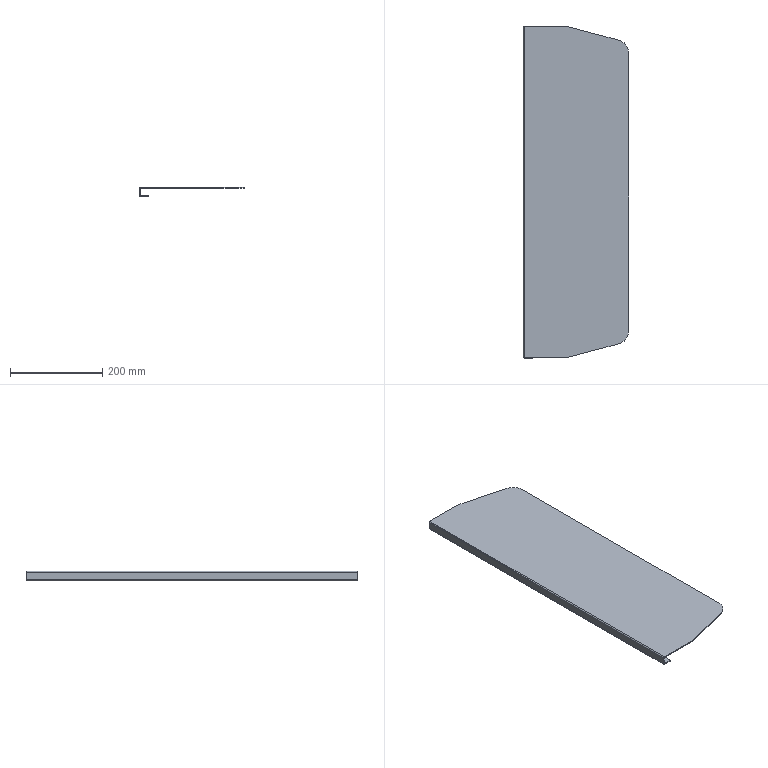Part | SolidWorks | features EdgeFlange 2, FlatPattern 1, SMBaseFlange 1, SheetMetal 1 | 1 solid | 26 faces | box 227.9 x 719 x 20 mm | volume 367716 mm3 | plane 20 | cylinder 6 | commonest cylinder face diameters 0.4 x2 4.4 x2 55.8 x2
STEP:
#1=CARTESIAN_POINT('',(2.,719.,-17.8));
#2=VERTEX_POINT('',#1);
#3=CARTESIAN_POINT('',(2.,719.,-2.2));
#4=VERTEX_POINT('',#3);
#5=CARTESIAN_POINT('',(2.,719.,0.));
#6=DIRECTION('',(0.,0.,1.));
#7=VECTOR('',#6,1000.);
#8=LINE('',#5,#7);
#9=EDGE_CURVE('',#2,#4,#8,.T.);
#10=ORIENTED_EDGE('',*,*,#9,.F.);
#11=CARTESIAN_POINT('',(0.,719.,-17.8));
#12=VERTEX_POINT('',#11);
#13=CARTESIAN_POINT('',(2.,719.,-17.8));
#14=DIRECTION('',(-1.,0.,0.));
#15=VECTOR('',#14,1000.);
#16=LINE('',#13,#15);
#17=EDGE_CURVE('',#2,#12,#16,.T.);
#18=ORIENTED_EDGE('',*,*,#17,.T.);
#19=CARTESIAN_POINT('',(0.,719.,-2.2));
#20=VERTEX_POINT('',#19);
#21=CARTESIAN_POINT('',(0.,719.,-2.));
#22=DIRECTION('',(0.,0.,1.));
#23=VECTOR('',#22,1000.);
#24=LINE('',#21,#23);
#25=EDGE_CURVE('',#12,#20,#24,.T.);
#26=ORIENTED_EDGE('',*,*,#25,.T.);
#27=CARTESIAN_POINT('',(2.,719.,-2.2));
#28=DIRECTION('',(-1.,0.,0.));
#29=VECTOR('',#28,1000.);
#30=LINE('',#27,#29);
#31=EDGE_CURVE('',#4,#20,#30,.T.);
#32=ORIENTED_EDGE('',*,*,#31,.F.);
#33=EDGE_LOOP('',(#10,#18,#26,#32));
#34=FACE_OUTER_BOUND('',#33,.T.);
#35=CARTESIAN_POINT('',(0.,719.,-2.));
#36=DIRECTION('',(0.,1.,0.));
#37=DIRECTION('',(0.,0.,1.));
#38=AXIS2_PLACEMENT_3D('',#35,#36,#37);
#39=PLANE('',#38);
#40=ADVANCED_FACE('',(#34),#39,.T.);
#41=ORIENTED_EDGE('',*,*,#25,.F.);
#42=CARTESIAN_POINT('',(0.,0.,-17.8));
#43=VERTEX_POINT('',#42);
#44=CARTESIAN_POINT('',(0.,719.,-17.8));
#45=DIRECTION('',(0.,-1.,0.));
#46=VECTOR('',#45,1000.);
#47=LINE('',#44,#46);
#48=EDGE_CURVE('',#12,#43,#47,.T.);
#49=ORIENTED_EDGE('',*,*,#48,.T.);
#50=CARTESIAN_POINT('',(0.,0.,-2.2));
#51=VERTEX_POINT('',#50);
#52=CARTESIAN_POINT('',(0.,0.,-20.));
#53=DIRECTION('',(0.,0.,-1.));
#54=VECTOR('',#53,1000.);
#55=LINE('',#52,#54);
#56=EDGE_CURVE('',#51,#43,#55,.T.);
#57=ORIENTED_EDGE('',*,*,#56,.F.);
#58=CARTESIAN_POINT('',(0.,0.,-2.2));
#59=DIRECTION('',(0.,1.,0.));
#60=VECTOR('',#59,1000.);
#61=LINE('',#58,#60);
#62=EDGE_CURVE('',#51,#20,#61,.T.);
#63=ORIENTED_EDGE('',*,*,#62,.T.);
#64=EDGE_LOOP('',(#41,#49,#57,#63));
#65=FACE_OUTER_BOUND('',#64,.T.);
#66=CARTESIAN_POINT('',(0.,0.,0.));
#67=DIRECTION('',(-1.,0.,0.));
#68=DIRECTION('',(0.,0.,1.));
#69=AXIS2_PLACEMENT_3D('',#66,#67,#68);
#70=PLANE('',#69);
#71=ADVANCED_FACE('',(#65),#70,.T.);
#72=CARTESIAN_POINT('',(2.,0.,-17.8));
#73=VERTEX_POINT('',#72);
#74=CARTESIAN_POINT('',(2.,719.,-17.8));
#75=DIRECTION('',(0.,-1.,0.));
#76=VECTOR('',#75,1000.);
#77=LINE('',#74,#76);
#78=EDGE_CURVE('',#2,#73,#77,.T.);
#79=ORIENTED_EDGE('',*,*,#78,.F.);
#80=ORIENTED_EDGE('',*,*,#9,.T.);
#81=CARTESIAN_POINT('',(2.,0.,-2.2));
#82=VERTEX_POINT('',#81);
#83=CARTESIAN_POINT('',(2.,0.,-2.2));
#84=DIRECTION('',(0.,1.,0.));
#85=VECTOR('',#84,1000.);
#86=LINE('',#83,#85);
#87=EDGE_CURVE('',#82,#4,#86,.T.);
#88=ORIENTED_EDGE('',*,*,#87,.F.);
#89=CARTESIAN_POINT('',(2.,0.,0.));
#90=DIRECTION('',(0.,0.,-1.));
#91=VECTOR('',#90,1000.);
#92=LINE('',#89,#91);
#93=EDGE_CURVE('',#82,#73,#92,.T.);
#94=ORIENTED_EDGE('',*,*,#93,.T.);
#95=EDGE_LOOP('',(#79,#80,#88,#94));
#96=FACE_OUTER_BOUND('',#95,.T.);
#97=CARTESIAN_POINT('',(2.,0.,0.));
#98=DIRECTION('',(-1.,0.,0.));
#99=DIRECTION('',(0.,0.,1.));
#100=AXIS2_PLACEMENT_3D('',#97,#98,#99);
#101=PLANE('',#100);
#102=ADVANCED_FACE('',(#96),#101,.F.);
#103=CARTESIAN_POINT('',(91.71,719.,-2.));
#104=VERTEX_POINT('',#103);
#105=CARTESIAN_POINT('',(2.2,719.,-2.));
#106=VERTEX_POINT('',#105);
#107=CARTESIAN_POINT('',(0.,719.,-2.));
#108=DIRECTION('',(-1.,0.,0.));
#109=VECTOR('',#108,1000.);
#110=LINE('',#107,#109);
#111=EDGE_CURVE('',#104,#106,#110,.T.);
#112=ORIENTED_EDGE('',*,*,#111,.T.);
#113=CARTESIAN_POINT('',(2.2,719.,0.));
#114=VERTEX_POINT('',#113);
#115=CARTESIAN_POINT('',(2.2,719.,-2.));
#116=DIRECTION('',(0.,0.,1.));
#117=VECTOR('',#116,1000.);
#118=LINE('',#115,#117);
#119=EDGE_CURVE('',#106,#114,#118,.T.);
#120=ORIENTED_EDGE('',*,*,#119,.T.);
#121=CARTESIAN_POINT('',(91.71,719.,0.));
#122=VERTEX_POINT('',#121);
#123=CARTESIAN_POINT('',(0.,719.,0.));
#124=DIRECTION('',(-1.,0.,0.));
#125=VECTOR('',#124,1000.);
#126=LINE('',#123,#125);
#127=EDGE_CURVE('',#122,#114,#126,.T.);
#128=ORIENTED_EDGE('',*,*,#127,.F.);
#129=CARTESIAN_POINT('',(91.71,719.,-2.));
#130=DIRECTION('',(0.,0.,1.));
#131=VECTOR('',#130,1000.);
#132=LINE('',#129,#131);
#133=EDGE_CURVE('',#104,#122,#132,.T.);
#134=ORIENTED_EDGE('',*,*,#133,.F.);
#135=EDGE_LOOP('',(#112,#120,#128,#134));
#136=FACE_OUTER_BOUND('',#135,.T.);
#137=CARTESIAN_POINT('',(0.,719.,-2.));
#138=DIRECTION('',(0.,1.,0.));
#139=DIRECTION('',(0.,0.,1.));
#140=AXIS2_PLACEMENT_3D('',#137,#138,#139);
#141=PLANE('',#140);
#142=ADVANCED_FACE('',(#136),#141,.T.);
#143=CARTESIAN_POINT('',(2.2,0.,-2.));
#144=VERTEX_POINT('',#143);
#145=CARTESIAN_POINT('',(91.71,0.,-2.));
#146=VERTEX_POINT('',#145);
#147=CARTESIAN_POINT('',(0.,0.,-2.));
#148=DIRECTION('',(1.,0.,0.));
#149=VECTOR('',#148,1000.);
#150=LINE('',#147,#149);
#151=EDGE_CURVE('',#144,#146,#150,.T.);
#152=ORIENTED_EDGE('',*,*,#151,.F.);
#153=CARTESIAN_POINT('',(2.2,719.,-2.));
#154=DIRECTION('',(0.,-1.,0.));
#155=VECTOR('',#154,1000.);
#156=LINE('',#153,#155);
#157=EDGE_CURVE('',#106,#144,#156,.T.);
#158=ORIENTED_EDGE('',*,*,#157,.F.);
#159=ORIENTED_EDGE('',*,*,#111,.F.);
#160=CARTESIAN_POINT('',(207.221,688.049,-2.));
#161=VERTEX_POINT('',#160);
#162=CARTESIAN_POINT('',(91.71,719.,-2.));
#163=DIRECTION('',(-0.9659,0.2588,0.));
#164=VECTOR('',#163,1000.);
#165=LINE('',#162,#164);
#166=EDGE_CURVE('',#161,#104,#165,.T.);
#167=ORIENTED_EDGE('',*,*,#166,.F.);
#168=CARTESIAN_POINT('',(227.9,661.1,-2.));
#169=VERTEX_POINT('',#168);
#170=CARTESIAN_POINT('',(200.,661.1,-2.));
#171=DIRECTION('',(0.,0.,1.));
#172=DIRECTION('',(1.,0.,0.));
#173=AXIS2_PLACEMENT_3D('',#170,#171,#172);
#174=CIRCLE('',#173,27.9);
#175=EDGE_CURVE('',#169,#161,#174,.T.);
#176=ORIENTED_EDGE('',*,*,#175,.F.);
#177=CARTESIAN_POINT('',(227.9,57.9,-2.));
#178=VERTEX_POINT('',#177);
#179=CARTESIAN_POINT('',(227.9,57.9,-2.));
#180=DIRECTION('',(0.,1.,0.));
#181=VECTOR('',#180,1000.);
#182=LINE('',#179,#181);
#183=EDGE_CURVE('',#178,#169,#182,.T.);
#184=ORIENTED_EDGE('',*,*,#183,.F.);
#185=CARTESIAN_POINT('',(207.221,30.951,-2.));
#186=VERTEX_POINT('',#185);
#187=CARTESIAN_POINT('',(200.,57.9,-2.));
#188=DIRECTION('',(0.,0.,1.));
#189=DIRECTION('',(-1.,0.,0.));
#190=AXIS2_PLACEMENT_3D('',#187,#188,#189);
#191=CIRCLE('',#190,27.9);
#192=EDGE_CURVE('',#186,#178,#191,.T.);
#193=ORIENTED_EDGE('',*,*,#192,.F.);
#194=CARTESIAN_POINT('',(91.71,0.,-2.));
#195=DIRECTION('',(0.9659,0.2588,0.));
#196=VECTOR('',#195,1000.);
#197=LINE('',#194,#196);
#198=EDGE_CURVE('',#146,#186,#197,.T.);
#199=ORIENTED_EDGE('',*,*,#198,.F.);
#200=EDGE_LOOP('',(#152,#158,#159,#167,#176,#184,#193,#199));
#201=FACE_OUTER_BOUND('',#200,.T.);
#202=CARTESIAN_POINT('',(200.,57.9,-2.));
#203=DIRECTION('',(0.,0.,-1.));
#204=DIRECTION('',(-1.,0.,0.));
#205=AXIS2_PLACEMENT_3D('',#202,#203,#204);
#206=PLANE('',#205);
#207=ADVANCED_FACE('',(#201),#206,.T.);
#208=CARTESIAN_POINT('',(2.2,0.,0.));
#209=VERTEX_POINT('',#208);
#210=CARTESIAN_POINT('',(2.2,719.,0.));
#211=DIRECTION('',(0.,-1.,0.));
#212=VECTOR('',#211,1000.);
#213=LINE('',#210,#212);
#214=EDGE_CURVE('',#114,#209,#213,.T.);
#215=ORIENTED_EDGE('',*,*,#214,.T.);
#216=CARTESIAN_POINT('',(91.71,0.,0.));
#217=VERTEX_POINT('',#216);
#218=CARTESIAN_POINT('',(0.,0.,0.));
#219=DIRECTION('',(1.,0.,0.));
#220=VECTOR('',#219,1000.);
#221=LINE('',#218,#220);
#222=EDGE_CURVE('',#209,#217,#221,.T.);
#223=ORIENTED_EDGE('',*,*,#222,.T.);
#224=CARTESIAN_POINT('',(207.221,30.951,0.));
#225=VERTEX_POINT('',#224);
#226=CARTESIAN_POINT('',(91.71,0.,0.));
#227=DIRECTION('',(0.9659,0.2588,0.));
#228=VECTOR('',#227,1000.);
#229=LINE('',#226,#228);
#230=EDGE_CURVE('',#217,#225,#229,.T.);
#231=ORIENTED_EDGE('',*,*,#230,.T.);
#232=CARTESIAN_POINT('',(227.9,57.9,0.));
#233=VERTEX_POINT('',#232);
#234=CARTESIAN_POINT('',(200.,57.9,0.));
#235=DIRECTION('',(0.,0.,1.));
#236=DIRECTION('',(-1.,0.,0.));
#237=AXIS2_PLACEMENT_3D('',#234,#235,#236);
#238=CIRCLE('',#237,27.9);
#239=EDGE_CURVE('',#225,#233,#238,.T.);
#240=ORIENTED_EDGE('',*,*,#239,.T.);
#241=CARTESIAN_POINT('',(227.9,661.1,0.));
#242=VERTEX_POINT('',#241);
#243=CARTESIAN_POINT('',(227.9,57.9,0.));
#244=DIRECTION('',(0.,1.,0.));
#245=VECTOR('',#244,1000.);
#246=LINE('',#243,#245);
#247=EDGE_CURVE('',#233,#242,#246,.T.);
#248=ORIENTED_EDGE('',*,*,#247,.T.);
#249=CARTESIAN_POINT('',(207.221,688.049,0.));
#250=VERTEX_POINT('',#249);
#251=CARTESIAN_POINT('',(200.,661.1,0.));
#252=DIRECTION('',(0.,0.,1.));
#253=DIRECTION('',(1.,0.,0.));
#254=AXIS2_PLACEMENT_3D('',#251,#252,#253);
#255=CIRCLE('',#254,27.9);
#256=EDGE_CURVE('',#242,#250,#255,.T.);
#257=ORIENTED_EDGE('',*,*,#256,.T.);
#258=CARTESIAN_POINT('',(91.71,719.,0.));
#259=DIRECTION('',(-0.9659,0.2588,0.));
#260=VECTOR('',#259,1000.);
#261=LINE('',#258,#260);
#262=EDGE_CURVE('',#250,#122,#261,.T.);
#263=ORIENTED_EDGE('',*,*,#262,.T.);
#264=ORIENTED_EDGE('',*,*,#127,.T.);
#265=EDGE_LOOP('',(#215,#223,#231,#240,#248,#257,#263,#264));
#266=FACE_OUTER_BOUND('',#265,.T.);
#267=CARTESIAN_POINT('',(200.,57.9,0.));
#268=DIRECTION('',(0.,0.,-1.));
#269=DIRECTION('',(-1.,0.,0.));
#270=AXIS2_PLACEMENT_3D('',#267,#268,#269);
#271=PLANE('',#270);
#272=ADVANCED_FACE('',(#266),#271,.F.);
#273=CARTESIAN_POINT('',(2.2,0.,-2.));
#274=DIRECTION('',(0.,0.,1.));
#275=VECTOR('',#274,1000.);
#276=LINE('',#273,#275);
#277=EDGE_CURVE('',#144,#209,#276,.T.);
#278=ORIENTED_EDGE('',*,*,#277,.F.);
#279=ORIENTED_EDGE('',*,*,#151,.T.);
#280=CARTESIAN_POINT('',(91.71,0.,-2.));
#281=DIRECTION('',(0.,0.,1.));
#282=VECTOR('',#281,1000.);
#283=LINE('',#280,#282);
#284=EDGE_CURVE('',#146,#217,#283,.T.);
#285=ORIENTED_EDGE('',*,*,#284,.T.);
#286=ORIENTED_EDGE('',*,*,#222,.F.);
#287=EDGE_LOOP('',(#278,#279,#285,#286));
#288=FACE_OUTER_BOUND('',#287,.T.);
#289=CARTESIAN_POINT('',(0.,0.,-2.));
#290=DIRECTION('',(0.,-1.,0.));
#291=DIRECTION('',(0.,0.,-1.));
#292=AXIS2_PLACEMENT_3D('',#289,#290,#291);
#293=PLANE('',#292);
#294=ADVANCED_FACE('',(#288),#293,.T.);
#295=ORIENTED_EDGE('',*,*,#262,.F.);
#296=CARTESIAN_POINT('',(207.221,688.049,-2.));
#297=DIRECTION('',(0.,0.,1.));
#298=VECTOR('',#297,1000.);
#299=LINE('',#296,#298);
#300=EDGE_CURVE('',#161,#250,#299,.T.);
#301=ORIENTED_EDGE('',*,*,#300,.F.);
#302=ORIENTED_EDGE('',*,*,#166,.T.);
#303=ORIENTED_EDGE('',*,*,#133,.T.);
#304=EDGE_LOOP('',(#295,#301,#302,#303));
#305=FACE_OUTER_BOUND('',#304,.T.);
#306=CARTESIAN_POINT('',(91.71,719.,-2.));
#307=DIRECTION('',(0.2588,0.9659,0.));
#308=DIRECTION('',(-0.9659,0.2588,0.));
#309=AXIS2_PLACEMENT_3D('',#306,#307,#308);
#310=PLANE('',#309);
#311=ADVANCED_FACE('',(#305),#310,.T.);
#312=ORIENTED_EDGE('',*,*,#256,.F.);
#313=CARTESIAN_POINT('',(227.9,661.1,-2.));
#314=DIRECTION('',(0.,0.,1.));
#315=VECTOR('',#314,1000.);
#316=LINE('',#313,#315);
#317=EDGE_CURVE('',#169,#242,#316,.T.);
#318=ORIENTED_EDGE('',*,*,#317,.F.);
#319=ORIENTED_EDGE('',*,*,#175,.T.);
#320=ORIENTED_EDGE('',*,*,#300,.T.);
#321=EDGE_LOOP('',(#312,#318,#319,#320));
#322=FACE_OUTER_BOUND('',#321,.T.);
#323=CARTESIAN_POINT('',(200.,661.1,-2.));
#324=DIRECTION('',(0.,0.,1.));
#325=DIRECTION('',(1.,0.,0.));
#326=AXIS2_PLACEMENT_3D('',#323,#324,#325);
#327=CYLINDRICAL_SURFACE('',#326,27.9);
#328=ADVANCED_FACE('',(#322),#327,.T.);
#329=ORIENTED_EDGE('',*,*,#247,.F.);
#330=CARTESIAN_POINT('',(227.9,57.9,-2.));
#331=DIRECTION('',(0.,0.,1.));
#332=VECTOR('',#331,1000.);
#333=LINE('',#330,#332);
#334=EDGE_CURVE('',#178,#233,#333,.T.);
#335=ORIENTED_EDGE('',*,*,#334,.F.);
#336=ORIENTED_EDGE('',*,*,#183,.T.);
#337=ORIENTED_EDGE('',*,*,#317,.T.);
#338=EDGE_LOOP('',(#329,#335,#336,#337));
#339=FACE_OUTER_BOUND('',#338,.T.);
#340=CARTESIAN_POINT('',(227.9,57.9,-2.));
#341=DIRECTION('',(1.,0.,0.));
#342=DIRECTION('',(0.,0.,-1.));
#343=AXIS2_PLACEMENT_3D('',#340,#341,#342);
#344=PLANE('',#343);
#345=ADVANCED_FACE('',(#339),#344,.T.);
#346=ORIENTED_EDGE('',*,*,#239,.F.);
#347=CARTESIAN_POINT('',(207.221,30.951,-2.));
#348=DIRECTION('',(0.,0.,1.));
#349=VECTOR('',#348,1000.);
#350=LINE('',#347,#349);
#351=EDGE_CURVE('',#186,#225,#350,.T.);
#352=ORIENTED_EDGE('',*,*,#351,.F.);
#353=ORIENTED_EDGE('',*,*,#192,.T.);
#354=ORIENTED_EDGE('',*,*,#334,.T.);
#355=EDGE_LOOP('',(#346,#352,#353,#354));
#356=FACE_OUTER_BOUND('',#355,.T.);
#357=CARTESIAN_POINT('',(200.,57.9,-2.));
#358=DIRECTION('',(0.,0.,1.));
#359=DIRECTION('',(1.,0.,0.));
#360=AXIS2_PLACEMENT_3D('',#357,#358,#359);
#361=CYLINDRICAL_SURFACE('',#360,27.9);
#362=ADVANCED_FACE('',(#356),#361,.T.);
#363=ORIENTED_EDGE('',*,*,#230,.F.);
#364=ORIENTED_EDGE('',*,*,#284,.F.);
#365=ORIENTED_EDGE('',*,*,#198,.T.);
#366=ORIENTED_EDGE('',*,*,#351,.T.);
#367=EDGE_LOOP('',(#363,#364,#365,#366));
#368=FACE_OUTER_BOUND('',#367,.T.);
#369=CARTESIAN_POINT('',(91.71,0.,-2.));
#370=DIRECTION('',(0.2588,-0.9659,0.));
#371=DIRECTION('',(0.9659,0.2588,0.));
#372=AXIS2_PLACEMENT_3D('',#369,#370,#371);
#373=PLANE('',#372);
#374=ADVANCED_FACE('',(#368),#373,.T.);
#375=CARTESIAN_POINT('',(0.,0.,-2.2));
#376=DIRECTION('',(-1.,0.,0.));
#377=VECTOR('',#376,1000.);
#378=LINE('',#375,#377);
#379=EDGE_CURVE('',#82,#51,#378,.T.);
#380=ORIENTED_EDGE('',*,*,#379,.F.);
#381=CARTESIAN_POINT('',(2.2,0.,-2.2));
#382=DIRECTION('',(0.,-1.,0.));
#383=DIRECTION('',(0.,0.,1.));
#384=AXIS2_PLACEMENT_3D('',#381,#382,#383);
#385=CIRCLE('',#384,0.2);
#386=EDGE_CURVE('',#144,#82,#385,.T.);
#387=ORIENTED_EDGE('',*,*,#386,.F.);
#388=ORIENTED_EDGE('',*,*,#277,.T.);
#389=CARTESIAN_POINT('',(2.2,0.,-2.2));
#390=DIRECTION('',(0.,-1.,0.));
#391=DIRECTION('',(0.,0.,1.));
#392=AXIS2_PLACEMENT_3D('',#389,#390,#391);
#393=CIRCLE('',#392,2.2);
#394=EDGE_CURVE('',#209,#51,#393,.T.);
#395=ORIENTED_EDGE('',*,*,#394,.T.);
#396=EDGE_LOOP('',(#380,#387,#388,#395));
#397=FACE_OUTER_BOUND('',#396,.T.);
#398=CARTESIAN_POINT('',(2.2,0.,-2.2));
#399=DIRECTION('',(0.,-1.,0.));
#400=DIRECTION('',(0.,0.,-1.));
#401=AXIS2_PLACEMENT_3D('',#398,#399,#400);
#402=PLANE('',#401);
#403=ADVANCED_FACE('',(#397),#402,.T.);
#404=CARTESIAN_POINT('',(2.2,719.,-2.2));
#405=DIRECTION('',(0.,1.,0.));
#406=DIRECTION('',(0.,0.,1.));
#407=AXIS2_PLACEMENT_3D('',#404,#405,#406);
#408=CIRCLE('',#407,0.2);
#409=EDGE_CURVE('',#4,#106,#408,.T.);
#410=ORIENTED_EDGE('',*,*,#409,.F.);
#411=ORIENTED_EDGE('',*,*,#31,.T.);
#412=CARTESIAN_POINT('',(2.2,719.,-2.2));
#413=DIRECTION('',(0.,1.,0.));
#414=DIRECTION('',(0.,0.,1.));
#415=AXIS2_PLACEMENT_3D('',#412,#413,#414);
#416=CIRCLE('',#415,2.2);
#417=EDGE_CURVE('',#20,#114,#416,.T.);
#418=ORIENTED_EDGE('',*,*,#417,.T.);
#419=ORIENTED_EDGE('',*,*,#119,.F.);
#420=EDGE_LOOP('',(#410,#411,#418,#419));
#421=FACE_OUTER_BOUND('',#420,.T.);
#422=CARTESIAN_POINT('',(2.2,719.,-2.2));
#423=DIRECTION('',(0.,-1.,0.));
#424=DIRECTION('',(0.,0.,-1.));
#425=AXIS2_PLACEMENT_3D('',#422,#423,#424);
#426=PLANE('',#425);
#427=ADVANCED_FACE('',(#421),#426,.F.);
#428=ORIENTED_EDGE('',*,*,#214,.F.);
#429=ORIENTED_EDGE('',*,*,#417,.F.);
#430=ORIENTED_EDGE('',*,*,#62,.F.);
#431=ORIENTED_EDGE('',*,*,#394,.F.);
#432=EDGE_LOOP('',(#428,#429,#430,#431));
#433=FACE_OUTER_BOUND('',#432,.T.);
#434=CARTESIAN_POINT('',(2.2,719.,-2.2));
#435=DIRECTION('',(0.,1.,0.));
#436=DIRECTION('',(-1.,0.,0.));
#437=AXIS2_PLACEMENT_3D('',#434,#435,#436);
#438=CYLINDRICAL_SURFACE('',#437,2.2);
#439=ADVANCED_FACE('',(#433),#438,.T.);
#440=ORIENTED_EDGE('',*,*,#157,.T.);
#441=ORIENTED_EDGE('',*,*,#386,.T.);
#442=ORIENTED_EDGE('',*,*,#87,.T.);
#443=ORIENTED_EDGE('',*,*,#409,.T.);
#444=EDGE_LOOP('',(#440,#441,#442,#443));
#445=FACE_OUTER_BOUND('',#444,.T.);
#446=CARTESIAN_POINT('',(2.2,719.,-2.2));
#447=DIRECTION('',(0.,1.,0.));
#448=DIRECTION('',(-1.,0.,0.));
#449=AXIS2_PLACEMENT_3D('',#446,#447,#448);
#450=CYLINDRICAL_SURFACE('',#449,0.2);
#451=ADVANCED_FACE('',(#445),#450,.F.);
#452=CARTESIAN_POINT('',(2.,0.,-17.8));
#453=DIRECTION('',(-1.,0.,0.));
#454=VECTOR('',#453,1000.);
#455=LINE('',#452,#454);
#456=EDGE_CURVE('',#73,#43,#455,.T.);
#457=ORIENTED_EDGE('',*,*,#456,.F.);
#458=ORIENTED_EDGE('',*,*,#93,.F.);
#459=ORIENTED_EDGE('',*,*,#379,.T.);
#460=ORIENTED_EDGE('',*,*,#56,.T.);
#461=EDGE_LOOP('',(#457,#458,#459,#460));
#462=FACE_OUTER_BOUND('',#461,.T.);
#463=CARTESIAN_POINT('',(0.,0.,-20.));
#464=DIRECTION('',(0.,-1.,0.));
#465=DIRECTION('',(0.,0.,-1.));
#466=AXIS2_PLACEMENT_3D('',#463,#464,#465);
#467=PLANE('',#466);
#468=ADVANCED_FACE('',(#462),#467,.T.);
#469=CARTESIAN_POINT('',(2.2,0.,-18.));
#470=VERTEX_POINT('',#469);
#471=CARTESIAN_POINT('',(2.2,0.,-20.));
#472=VERTEX_POINT('',#471);
#473=CARTESIAN_POINT('',(2.2,0.,-20.));
#474=DIRECTION('',(0.,0.,-1.));
#475=VECTOR('',#474,1000.);
#476=LINE('',#473,#475);
#477=EDGE_CURVE('',#470,#472,#476,.T.);
#478=ORIENTED_EDGE('',*,*,#477,.F.);
#479=CARTESIAN_POINT('',(2.2,0.,-17.8));
#480=DIRECTION('',(0.,-1.,0.));
#481=DIRECTION('',(0.,0.,1.));
#482=AXIS2_PLACEMENT_3D('',#479,#480,#481);
#483=CIRCLE('',#482,0.2);
#484=EDGE_CURVE('',#73,#470,#483,.T.);
#485=ORIENTED_EDGE('',*,*,#484,.F.);
#486=ORIENTED_EDGE('',*,*,#456,.T.);
#487=CARTESIAN_POINT('',(2.2,0.,-17.8));
#488=DIRECTION('',(0.,-1.,0.));
#489=DIRECTION('',(0.,0.,1.));
#490=AXIS2_PLACEMENT_3D('',#487,#488,#489);
#491=CIRCLE('',#490,2.2);
#492=EDGE_CURVE('',#43,#472,#491,.T.);
#493=ORIENTED_EDGE('',*,*,#492,.T.);
#494=EDGE_LOOP('',(#478,#485,#486,#493));
#495=FACE_OUTER_BOUND('',#494,.T.);
#496=CARTESIAN_POINT('',(2.2,0.,-17.8));
#497=DIRECTION('',(0.,-1.,0.));
#498=DIRECTION('',(0.,0.,-1.));
#499=AXIS2_PLACEMENT_3D('',#496,#497,#498);
#500=PLANE('',#499);
#501=ADVANCED_FACE('',(#495),#500,.T.);
#502=CARTESIAN_POINT('',(2.2,719.,-18.));
#503=VERTEX_POINT('',#502);
#504=CARTESIAN_POINT('',(2.2,719.,-17.8));
#505=DIRECTION('',(0.,1.,0.));
#506=DIRECTION('',(0.,0.,1.));
#507=AXIS2_PLACEMENT_3D('',#504,#505,#506);
#508=CIRCLE('',#507,0.2);
#509=EDGE_CURVE('',#503,#2,#508,.T.);
#510=ORIENTED_EDGE('',*,*,#509,.F.);
#511=CARTESIAN_POINT('',(2.2,719.,-20.));
#512=VERTEX_POINT('',#511);
#513=CARTESIAN_POINT('',(2.2,719.,-18.));
#514=DIRECTION('',(0.,0.,-1.));
#515=VECTOR('',#514,1000.);
#516=LINE('',#513,#515);
#517=EDGE_CURVE('',#503,#512,#516,.T.);
#518=ORIENTED_EDGE('',*,*,#517,.T.);
#519=CARTESIAN_POINT('',(2.2,719.,-17.8));
#520=DIRECTION('',(0.,1.,0.));
#521=DIRECTION('',(0.,0.,1.));
#522=AXIS2_PLACEMENT_3D('',#519,#520,#521);
#523=CIRCLE('',#522,2.2);
#524=EDGE_CURVE('',#512,#12,#523,.T.);
#525=ORIENTED_EDGE('',*,*,#524,.T.);
#526=ORIENTED_EDGE('',*,*,#17,.F.);
#527=EDGE_LOOP('',(#510,#518,#525,#526));
#528=FACE_OUTER_BOUND('',#527,.T.);
#529=CARTESIAN_POINT('',(2.2,719.,-17.8));
#530=DIRECTION('',(0.,-1.,0.));
#531=DIRECTION('',(0.,0.,-1.));
#532=AXIS2_PLACEMENT_3D('',#529,#530,#531);
#533=PLANE('',#532);
#534=ADVANCED_FACE('',(#528),#533,.F.);
#535=ORIENTED_EDGE('',*,*,#48,.F.);
#536=ORIENTED_EDGE('',*,*,#524,.F.);
#537=CARTESIAN_POINT('',(2.2,0.,-20.));
#538=DIRECTION('',(0.,1.,0.));
#539=VECTOR('',#538,1000.);
#540=LINE('',#537,#539);
#541=EDGE_CURVE('',#472,#512,#540,.T.);
#542=ORIENTED_EDGE('',*,*,#541,.F.);
#543=ORIENTED_EDGE('',*,*,#492,.F.);
#544=EDGE_LOOP('',(#535,#536,#542,#543));
#545=FACE_OUTER_BOUND('',#544,.T.);
#546=CARTESIAN_POINT('',(2.2,719.,-17.8));
#547=DIRECTION('',(0.,1.,0.));
#548=DIRECTION('',(0.,0.,-1.));
#549=AXIS2_PLACEMENT_3D('',#546,#547,#548);
#550=CYLINDRICAL_SURFACE('',#549,2.2);
#551=ADVANCED_FACE('',(#545),#550,.T.);
#552=ORIENTED_EDGE('',*,*,#78,.T.);
#553=ORIENTED_EDGE('',*,*,#484,.T.);
#554=CARTESIAN_POINT('',(2.2,0.,-18.));
#555=DIRECTION('',(0.,1.,0.));
#556=VECTOR('',#555,1000.);
#557=LINE('',#554,#556);
#558=EDGE_CURVE('',#470,#503,#557,.T.);
#559=ORIENTED_EDGE('',*,*,#558,.T.);
#560=ORIENTED_EDGE('',*,*,#509,.T.);
#561=EDGE_LOOP('',(#552,#553,#559,#560));
#562=FACE_OUTER_BOUND('',#561,.T.);
#563=CARTESIAN_POINT('',(2.2,719.,-17.8));
#564=DIRECTION('',(0.,1.,0.));
#565=DIRECTION('',(0.,0.,-1.));
#566=AXIS2_PLACEMENT_3D('',#563,#564,#565);
#567=CYLINDRICAL_SURFACE('',#566,0.2);
#568=ADVANCED_FACE('',(#562),#567,.F.);
#569=CARTESIAN_POINT('',(20.,719.,-20.));
#570=VERTEX_POINT('',#569);
#571=CARTESIAN_POINT('',(2.,719.,-20.));
#572=DIRECTION('',(-1.,0.,0.));
#573=VECTOR('',#572,1000.);
#574=LINE('',#571,#573);
#575=EDGE_CURVE('',#570,#512,#574,.T.);
#576=ORIENTED_EDGE('',*,*,#575,.T.);
#577=ORIENTED_EDGE('',*,*,#517,.F.);
#578=CARTESIAN_POINT('',(20.,719.,-18.));
#579=VERTEX_POINT('',#578);
#580=CARTESIAN_POINT('',(0.,719.,-18.));
#581=DIRECTION('',(-1.,0.,0.));
#582=VECTOR('',#581,1000.);
#583=LINE('',#580,#582);
#584=EDGE_CURVE('',#579,#503,#583,.T.);
#585=ORIENTED_EDGE('',*,*,#584,.F.);
#586=CARTESIAN_POINT('',(20.,719.,-20.));
#587=DIRECTION('',(0.,0.,1.));
#588=VECTOR('',#587,1000.);
#589=LINE('',#586,#588);
#590=EDGE_CURVE('',#570,#579,#589,.T.);
#591=ORIENTED_EDGE('',*,*,#590,.F.);
#592=EDGE_LOOP('',(#576,#577,#585,#591));
#593=FACE_OUTER_BOUND('',#592,.T.);
#594=CARTESIAN_POINT('',(2.,719.,-20.));
#595=DIRECTION('',(0.,1.,0.));
#596=DIRECTION('',(0.,0.,1.));
#597=AXIS2_PLACEMENT_3D('',#594,#595,#596);
#598=PLANE('',#597);
#599=ADVANCED_FACE('',(#593),#598,.T.);
#600=CARTESIAN_POINT('',(20.,0.,-18.));
#601=VERTEX_POINT('',#600);
#602=CARTESIAN_POINT('',(0.,0.,-18.));
#603=DIRECTION('',(1.,0.,0.));
#604=VECTOR('',#603,1000.);
#605=LINE('',#602,#604);
#606=EDGE_CURVE('',#470,#601,#605,.T.);
#607=ORIENTED_EDGE('',*,*,#606,.F.);
#608=ORIENTED_EDGE('',*,*,#477,.T.);
#609=CARTESIAN_POINT('',(20.,0.,-20.));
#610=VERTEX_POINT('',#609);
#611=CARTESIAN_POINT('',(20.,0.,-20.));
#612=DIRECTION('',(1.,0.,0.));
#613=VECTOR('',#612,1000.);
#614=LINE('',#611,#613);
#615=EDGE_CURVE('',#472,#610,#614,.T.);
#616=ORIENTED_EDGE('',*,*,#615,.T.);
#617=CARTESIAN_POINT('',(20.,0.,-20.));
#618=DIRECTION('',(0.,0.,1.));
#619=VECTOR('',#618,1000.);
#620=LINE('',#617,#619);
#621=EDGE_CURVE('',#610,#601,#620,.T.);
#622=ORIENTED_EDGE('',*,*,#621,.T.);
#623=EDGE_LOOP('',(#607,#608,#616,#622));
#624=FACE_OUTER_BOUND('',#623,.T.);
#625=CARTESIAN_POINT('',(20.,0.,-20.));
#626=DIRECTION('',(0.,-1.,0.));
#627=DIRECTION('',(0.,0.,-1.));
#628=AXIS2_PLACEMENT_3D('',#625,#626,#627);
#629=PLANE('',#628);
#630=ADVANCED_FACE('',(#624),#629,.T.);
#631=ORIENTED_EDGE('',*,*,#615,.F.);
#632=ORIENTED_EDGE('',*,*,#541,.T.);
#633=ORIENTED_EDGE('',*,*,#575,.F.);
#634=CARTESIAN_POINT('',(20.,719.,-20.));
#635=DIRECTION('',(0.,1.,0.));
#636=VECTOR('',#635,1000.);
#637=LINE('',#634,#636);
#638=EDGE_CURVE('',#610,#570,#637,.T.);
#639=ORIENTED_EDGE('',*,*,#638,.F.);
#640=EDGE_LOOP('',(#631,#632,#633,#639));
#641=FACE_OUTER_BOUND('',#640,.T.);
#642=CARTESIAN_POINT('',(0.,0.,-20.));
#643=DIRECTION('',(0.,0.,-1.));
#644=DIRECTION('',(-1.,0.,0.));
#645=AXIS2_PLACEMENT_3D('',#642,#643,#644);
#646=PLANE('',#645);
#647=ADVANCED_FACE('',(#641),#646,.T.);
#648=ORIENTED_EDGE('',*,*,#558,.F.);
#649=ORIENTED_EDGE('',*,*,#606,.T.);
#650=CARTESIAN_POINT('',(20.,0.,-18.));
#651=DIRECTION('',(0.,1.,0.));
#652=VECTOR('',#651,1000.);
#653=LINE('',#650,#652);
#654=EDGE_CURVE('',#601,#579,#653,.T.);
#655=ORIENTED_EDGE('',*,*,#654,.T.);
#656=ORIENTED_EDGE('',*,*,#584,.T.);
#657=EDGE_LOOP('',(#648,#649,#655,#656));
#658=FACE_OUTER_BOUND('',#657,.T.);
#659=CARTESIAN_POINT('',(0.,0.,-18.));
#660=DIRECTION('',(0.,0.,-1.));
#661=DIRECTION('',(-1.,0.,0.));
#662=AXIS2_PLACEMENT_3D('',#659,#660,#661);
#663=PLANE('',#662);
#664=ADVANCED_FACE('',(#658),#663,.F.);
#665=ORIENTED_EDGE('',*,*,#654,.F.);
#666=ORIENTED_EDGE('',*,*,#621,.F.);
#667=ORIENTED_EDGE('',*,*,#638,.T.);
#668=ORIENTED_EDGE('',*,*,#590,.T.);
#669=EDGE_LOOP('',(#665,#666,#667,#668));
#670=FACE_OUTER_BOUND('',#669,.T.);
#671=CARTESIAN_POINT('',(20.,719.,-20.));
#672=DIRECTION('',(1.,0.,0.));
#673=DIRECTION('',(0.,0.,-1.));
#674=AXIS2_PLACEMENT_3D('',#671,#672,#673);
#675=PLANE('',#674);
#676=ADVANCED_FACE('',(#670),#675,.T.);
#677=CLOSED_SHELL('',(#40,#71,#102,#142,#207,#272,#294,#311,#328,#345,#362,#374,#403,#427,#439,#451,#468,#501,#534,#551,#568,#599,#630,#647,#664,#676));
#678=MANIFOLD_SOLID_BREP('',#677);
#679=CARTESIAN_POINT('',(0.,0.,0.));
#680=DIRECTION('',(0.,0.,1.));
#681=DIRECTION('',(1.,0.,0.));
#682=AXIS2_PLACEMENT_3D('',#679,#680,#681);
#683=(LENGTH_UNIT()NAMED_UNIT(*)SI_UNIT(.MILLI.,.METRE.));
#684=UNCERTAINTY_MEASURE_WITH_UNIT(LENGTH_MEASURE(0.00001),#683,'','');
#685=(NAMED_UNIT(*)PLANE_ANGLE_UNIT()SI_UNIT($,.RADIAN.));
#686=(NAMED_UNIT(*)SI_UNIT($,.STERADIAN.)SOLID_ANGLE_UNIT());
#687=(GEOMETRIC_REPRESENTATION_CONTEXT(3)GLOBAL_UNCERTAINTY_ASSIGNED_CONTEXT((#684))GLOBAL_UNIT_ASSIGNED_CONTEXT((#683,#685,#686))REPRESENTATION_CONTEXT('',''));
#688=ADVANCED_BREP_SHAPE_REPRESENTATION('',(#678,#682),#687);